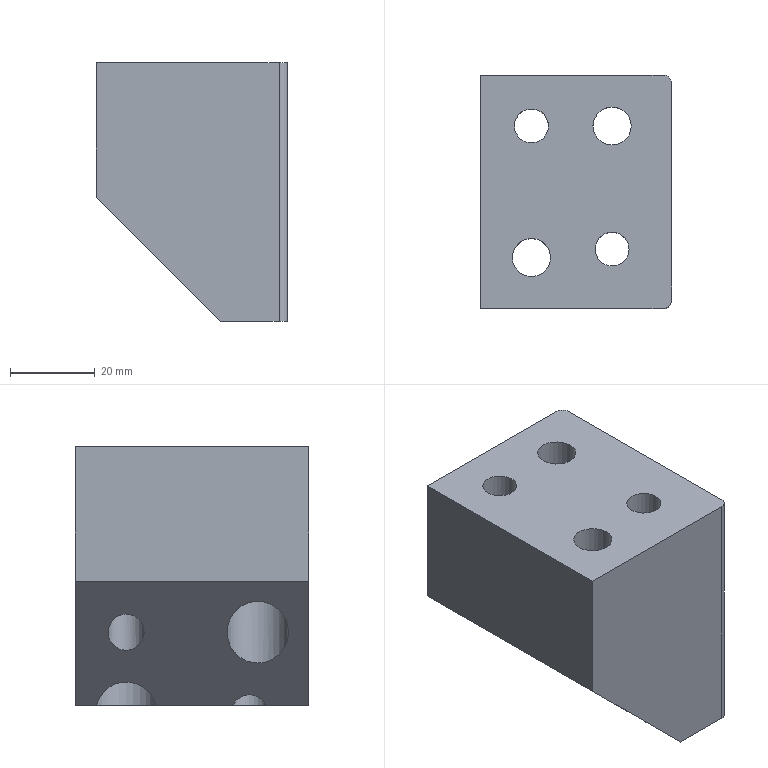Part | NX | features solid 2 | 1 solid | 21 faces | box 45 x 55 x 61 mm | volume 109585 mm3 | plane 11 | cylinder 10 | commonest cylinder face diameters 4 x2 8.001 x2 8.5 x2 9 x2 14.5 x2
STEP:
#1=CARTESIAN_POINT('',(620.135,-72.389,-6.));
#2=VERTEX_POINT('',#1);
#3=CARTESIAN_POINT('',(620.135,-80.141,-6.));
#4=VERTEX_POINT('',#3);
#5=CARTESIAN_POINT('',(621.878,-76.265,-6.));
#6=DIRECTION('',(0.,0.,1.));
#7=DIRECTION('',(1.,0.,0.));
#8=AXIS2_PLACEMENT_3D('',#5,#6,#7);
#9=CIRCLE('',#8,4.25);
#10=EDGE_CURVE('',#2,#4,#9,.F.);
#11=ORIENTED_EDGE('',*,*,#10,.F.);
#12=CARTESIAN_POINT('',(620.135,-54.303,-6.));
#13=VERTEX_POINT('',#12);
#14=CARTESIAN_POINT('',(620.135,88.864,-6.));
#15=DIRECTION('',(0.,1.,0.));
#16=VECTOR('',#15,1000.);
#17=LINE('',#14,#16);
#18=EDGE_CURVE('',#2,#13,#17,.T.);
#19=ORIENTED_EDGE('',*,*,#18,.T.);
#20=CARTESIAN_POINT('',(620.135,-40.228,-6.));
#21=VERTEX_POINT('',#20);
#22=CARTESIAN_POINT('',(621.878,-47.265,-6.));
#23=DIRECTION('',(0.,0.,-1.));
#24=DIRECTION('',(1.,0.,0.));
#25=AXIS2_PLACEMENT_3D('',#22,#23,#24);
#26=CIRCLE('',#25,7.25);
#27=EDGE_CURVE('',#13,#21,#26,.F.);
#28=ORIENTED_EDGE('',*,*,#27,.T.);
#29=CARTESIAN_POINT('',(620.135,-35.265,-6.));
#30=VERTEX_POINT('',#29);
#31=CARTESIAN_POINT('',(620.135,88.864,-6.));
#32=DIRECTION('',(0.,1.,0.));
#33=VECTOR('',#32,1000.);
#34=LINE('',#31,#33);
#35=EDGE_CURVE('',#21,#30,#34,.T.);
#36=ORIENTED_EDGE('',*,*,#35,.T.);
#37=CARTESIAN_POINT('',(633.878,-35.265,-6.));
#38=VERTEX_POINT('',#37);
#39=CARTESIAN_POINT('',(735.,-35.265,-6.));
#40=DIRECTION('',(-1.,0.,0.));
#41=VECTOR('',#40,1000.);
#42=LINE('',#39,#41);
#43=EDGE_CURVE('',#30,#38,#42,.F.);
#44=ORIENTED_EDGE('',*,*,#43,.T.);
#45=CARTESIAN_POINT('',(635.878,-37.265,-6.));
#46=VERTEX_POINT('',#45);
#47=CARTESIAN_POINT('',(633.878,-37.265,-6.));
#48=DIRECTION('',(0.,0.,1.));
#49=DIRECTION('',(1.,0.,0.));
#50=AXIS2_PLACEMENT_3D('',#47,#48,#49);
#51=CIRCLE('',#50,2.);
#52=EDGE_CURVE('',#46,#38,#51,.T.);
#53=ORIENTED_EDGE('',*,*,#52,.F.);
#54=CARTESIAN_POINT('',(635.878,-88.265,-6.));
#55=VERTEX_POINT('',#54);
#56=CARTESIAN_POINT('',(635.878,-52.29,-6.));
#57=DIRECTION('',(0.,1.,0.));
#58=VECTOR('',#57,1000.);
#59=LINE('',#56,#58);
#60=EDGE_CURVE('',#46,#55,#59,.F.);
#61=ORIENTED_EDGE('',*,*,#60,.T.);
#62=CARTESIAN_POINT('',(633.878,-90.265,-6.));
#63=VERTEX_POINT('',#62);
#64=CARTESIAN_POINT('',(633.878,-88.265,-6.));
#65=DIRECTION('',(0.,0.,1.));
#66=DIRECTION('',(1.,0.,0.));
#67=AXIS2_PLACEMENT_3D('',#64,#65,#66);
#68=CIRCLE('',#67,2.);
#69=EDGE_CURVE('',#55,#63,#68,.F.);
#70=ORIENTED_EDGE('',*,*,#69,.T.);
#71=CARTESIAN_POINT('',(620.135,-90.265,-6.));
#72=VERTEX_POINT('',#71);
#73=CARTESIAN_POINT('',(735.,-90.265,-6.));
#74=DIRECTION('',(1.,0.,0.));
#75=VECTOR('',#74,1000.);
#76=LINE('',#73,#75);
#77=EDGE_CURVE('',#63,#72,#76,.F.);
#78=ORIENTED_EDGE('',*,*,#77,.T.);
#79=CARTESIAN_POINT('',(620.135,88.864,-6.));
#80=DIRECTION('',(0.,1.,0.));
#81=VECTOR('',#80,1000.);
#82=LINE('',#79,#81);
#83=EDGE_CURVE('',#72,#4,#82,.T.);
#84=ORIENTED_EDGE('',*,*,#83,.T.);
#85=EDGE_LOOP('',(#11,#19,#28,#36,#44,#53,#61,#70,#78,#84));
#86=FACE_BOUND('',#85,.T.);
#87=CARTESIAN_POINT('',(735.,88.864,-6.));
#88=DIRECTION('',(0.,0.,1.));
#89=DIRECTION('',(-0.9997,0.02352,0.));
#90=AXIS2_PLACEMENT_3D('',#87,#88,#89);
#91=PLANE('',#90);
#92=ADVANCED_FACE('',(#86),#91,.F.);
#93=CARTESIAN_POINT('',(590.878,-90.265,23.257));
#94=VERTEX_POINT('',#93);
#95=CARTESIAN_POINT('',(590.878,-90.265,55.));
#96=VERTEX_POINT('',#95);
#97=CARTESIAN_POINT('',(590.878,-90.265,-5.));
#98=DIRECTION('',(0.,0.,1.));
#99=VECTOR('',#98,1000.);
#100=LINE('',#97,#99);
#101=EDGE_CURVE('',#94,#96,#100,.T.);
#102=ORIENTED_EDGE('',*,*,#101,.T.);
#103=CARTESIAN_POINT('',(590.878,-35.265,55.));
#104=VERTEX_POINT('',#103);
#105=CARTESIAN_POINT('',(590.878,-52.29,55.));
#106=DIRECTION('',(0.,1.,0.));
#107=VECTOR('',#106,1000.);
#108=LINE('',#105,#107);
#109=EDGE_CURVE('',#96,#104,#108,.T.);
#110=ORIENTED_EDGE('',*,*,#109,.T.);
#111=CARTESIAN_POINT('',(590.878,-35.265,23.257));
#112=VERTEX_POINT('',#111);
#113=CARTESIAN_POINT('',(590.878,-35.265,-5.));
#114=DIRECTION('',(0.,0.,1.));
#115=VECTOR('',#114,1000.);
#116=LINE('',#113,#115);
#117=EDGE_CURVE('',#112,#104,#116,.T.);
#118=ORIENTED_EDGE('',*,*,#117,.F.);
#119=CARTESIAN_POINT('',(590.878,-52.29,23.257));
#120=DIRECTION('',(0.,-1.,0.));
#121=VECTOR('',#120,1000.);
#122=LINE('',#119,#121);
#123=EDGE_CURVE('',#94,#112,#122,.F.);
#124=ORIENTED_EDGE('',*,*,#123,.F.);
#125=EDGE_LOOP('',(#102,#110,#118,#124));
#126=FACE_BOUND('',#125,.T.);
#127=CARTESIAN_POINT('',(590.878,-52.29,-5.));
#128=DIRECTION('',(-1.,0.,0.));
#129=DIRECTION('',(0.,0.,1.));
#130=AXIS2_PLACEMENT_3D('',#127,#128,#129);
#131=PLANE('',#130);
#132=ADVANCED_FACE('',(#126),#131,.T.);
#133=CARTESIAN_POINT('',(635.878,-37.265,55.));
#134=VERTEX_POINT('',#133);
#135=CARTESIAN_POINT('',(635.878,-37.265,-5.));
#136=DIRECTION('',(0.,0.,1.));
#137=VECTOR('',#136,1000.);
#138=LINE('',#135,#137);
#139=EDGE_CURVE('',#134,#46,#138,.F.);
#140=ORIENTED_EDGE('',*,*,#139,.F.);
#141=CARTESIAN_POINT('',(635.878,-88.265,55.));
#142=VERTEX_POINT('',#141);
#143=CARTESIAN_POINT('',(635.878,-52.29,55.));
#144=DIRECTION('',(0.,-1.,0.));
#145=VECTOR('',#144,1000.);
#146=LINE('',#143,#145);
#147=EDGE_CURVE('',#134,#142,#146,.T.);
#148=ORIENTED_EDGE('',*,*,#147,.T.);
#149=CARTESIAN_POINT('',(635.878,-88.265,-5.));
#150=DIRECTION('',(0.,0.,-1.));
#151=VECTOR('',#150,1000.);
#152=LINE('',#149,#151);
#153=EDGE_CURVE('',#142,#55,#152,.T.);
#154=ORIENTED_EDGE('',*,*,#153,.T.);
#155=ORIENTED_EDGE('',*,*,#60,.F.);
#156=EDGE_LOOP('',(#140,#148,#154,#155));
#157=FACE_BOUND('',#156,.T.);
#158=CARTESIAN_POINT('',(635.878,-52.29,-5.));
#159=DIRECTION('',(1.,0.,0.));
#160=DIRECTION('',(0.,0.,-1.));
#161=AXIS2_PLACEMENT_3D('',#158,#159,#160);
#162=PLANE('',#161);
#163=ADVANCED_FACE('',(#157),#162,.T.);
#164=ORIENTED_EDGE('',*,*,#117,.T.);
#165=CARTESIAN_POINT('',(633.878,-35.265,55.));
#166=VERTEX_POINT('',#165);
#167=CARTESIAN_POINT('',(630.878,-35.265,55.));
#168=DIRECTION('',(1.,0.,0.));
#169=VECTOR('',#168,1000.);
#170=LINE('',#167,#169);
#171=EDGE_CURVE('',#104,#166,#170,.T.);
#172=ORIENTED_EDGE('',*,*,#171,.T.);
#173=CARTESIAN_POINT('',(633.878,-35.265,-5.));
#174=DIRECTION('',(0.,0.,1.));
#175=VECTOR('',#174,1000.);
#176=LINE('',#173,#175);
#177=EDGE_CURVE('',#38,#166,#176,.T.);
#178=ORIENTED_EDGE('',*,*,#177,.F.);
#179=ORIENTED_EDGE('',*,*,#43,.F.);
#180=CARTESIAN_POINT('',(613.756,-35.265,0.3787));
#181=DIRECTION('',(-0.7071,0.,0.7071));
#182=VECTOR('',#181,1000.);
#183=LINE('',#180,#182);
#184=EDGE_CURVE('',#112,#30,#183,.F.);
#185=ORIENTED_EDGE('',*,*,#184,.F.);
#186=EDGE_LOOP('',(#164,#172,#178,#179,#185));
#187=FACE_BOUND('',#186,.T.);
#188=CARTESIAN_POINT('',(630.878,-35.265,-5.));
#189=DIRECTION('',(0.,1.,0.));
#190=DIRECTION('',(0.,0.,1.));
#191=AXIS2_PLACEMENT_3D('',#188,#189,#190);
#192=PLANE('',#191);
#193=ADVANCED_FACE('',(#187),#192,.T.);
#194=ORIENTED_EDGE('',*,*,#177,.T.);
#195=CARTESIAN_POINT('',(633.878,-37.265,55.));
#196=DIRECTION('',(0.,0.,1.));
#197=DIRECTION('',(1.,0.,0.));
#198=AXIS2_PLACEMENT_3D('',#195,#196,#197);
#199=CIRCLE('',#198,2.);
#200=EDGE_CURVE('',#166,#134,#199,.F.);
#201=ORIENTED_EDGE('',*,*,#200,.T.);
#202=ORIENTED_EDGE('',*,*,#139,.T.);
#203=ORIENTED_EDGE('',*,*,#52,.T.);
#204=EDGE_LOOP('',(#194,#201,#202,#203));
#205=FACE_BOUND('',#204,.T.);
#206=CARTESIAN_POINT('',(633.878,-37.265,-5.));
#207=DIRECTION('',(0.,0.,-1.));
#208=DIRECTION('',(-1.,0.,0.));
#209=AXIS2_PLACEMENT_3D('',#206,#207,#208);
#210=CYLINDRICAL_SURFACE('',#209,2.);
#211=ADVANCED_FACE('',(#205),#210,.T.);
#212=CARTESIAN_POINT('',(633.878,-90.265,55.));
#213=VERTEX_POINT('',#212);
#214=CARTESIAN_POINT('',(633.878,-90.265,22.));
#215=DIRECTION('',(0.,0.,-1.));
#216=VECTOR('',#215,1000.);
#217=LINE('',#214,#216);
#218=EDGE_CURVE('',#63,#213,#217,.F.);
#219=ORIENTED_EDGE('',*,*,#218,.T.);
#220=CARTESIAN_POINT('',(619.878,-90.265,55.));
#221=DIRECTION('',(-1.,0.,0.));
#222=VECTOR('',#221,1000.);
#223=LINE('',#220,#222);
#224=EDGE_CURVE('',#213,#96,#223,.T.);
#225=ORIENTED_EDGE('',*,*,#224,.T.);
#226=ORIENTED_EDGE('',*,*,#101,.F.);
#227=CARTESIAN_POINT('',(613.756,-90.265,0.3787));
#228=DIRECTION('',(0.7071,0.,-0.7071));
#229=VECTOR('',#228,1000.);
#230=LINE('',#227,#229);
#231=EDGE_CURVE('',#72,#94,#230,.F.);
#232=ORIENTED_EDGE('',*,*,#231,.F.);
#233=ORIENTED_EDGE('',*,*,#77,.F.);
#234=EDGE_LOOP('',(#219,#225,#226,#232,#233));
#235=FACE_BOUND('',#234,.T.);
#236=CARTESIAN_POINT('',(619.878,-90.265,22.));
#237=DIRECTION('',(0.,-1.,0.));
#238=DIRECTION('',(0.,0.,-1.));
#239=AXIS2_PLACEMENT_3D('',#236,#237,#238);
#240=PLANE('',#239);
#241=ADVANCED_FACE('',(#235),#240,.T.);
#242=ORIENTED_EDGE('',*,*,#153,.F.);
#243=CARTESIAN_POINT('',(633.878,-88.265,55.));
#244=DIRECTION('',(0.,0.,1.));
#245=DIRECTION('',(1.,0.,0.));
#246=AXIS2_PLACEMENT_3D('',#243,#244,#245);
#247=CIRCLE('',#246,2.);
#248=EDGE_CURVE('',#142,#213,#247,.F.);
#249=ORIENTED_EDGE('',*,*,#248,.T.);
#250=ORIENTED_EDGE('',*,*,#218,.F.);
#251=ORIENTED_EDGE('',*,*,#69,.F.);
#252=EDGE_LOOP('',(#242,#249,#250,#251));
#253=FACE_BOUND('',#252,.T.);
#254=CARTESIAN_POINT('',(633.878,-88.265,-5.));
#255=DIRECTION('',(0.,0.,-1.));
#256=DIRECTION('',(-1.,0.,0.));
#257=AXIS2_PLACEMENT_3D('',#254,#255,#256);
#258=CYLINDRICAL_SURFACE('',#257,2.);
#259=ADVANCED_FACE('',(#253),#258,.T.);
#260=CARTESIAN_POINT('',(598.628,-47.265,15.507));
#261=VERTEX_POINT('',#260);
#262=CARTESIAN_POINT('',(602.878,-47.265,11.257));
#263=DIRECTION('',(0.7071,0.,0.7071));
#264=DIRECTION('',(-0.7071,0.,0.7071));
#265=AXIS2_PLACEMENT_3D('',#262,#263,#264);
#266=ELLIPSE('',#265,6.01,4.25);
#267=EDGE_CURVE('',#261,#261,#266,.F.);
#268=ORIENTED_EDGE('',*,*,#267,.F.);
#269=EDGE_LOOP('',(#268));
#270=FACE_BOUND('',#269,.T.);
#271=CARTESIAN_POINT('',(621.878,-76.265,-7.743));
#272=DIRECTION('',(0.7071,0.,0.7071));
#273=DIRECTION('',(-0.7071,0.,0.7071));
#274=AXIS2_PLACEMENT_3D('',#271,#272,#273);
#275=ELLIPSE('',#274,6.01,4.25);
#276=EDGE_CURVE('',#4,#2,#275,.F.);
#277=ORIENTED_EDGE('',*,*,#276,.F.);
#278=ORIENTED_EDGE('',*,*,#83,.F.);
#279=ORIENTED_EDGE('',*,*,#231,.T.);
#280=ORIENTED_EDGE('',*,*,#123,.T.);
#281=ORIENTED_EDGE('',*,*,#184,.T.);
#282=ORIENTED_EDGE('',*,*,#35,.F.);
#283=CARTESIAN_POINT('',(621.878,-47.265,-7.743));
#284=DIRECTION('',(0.7071,0.,0.7071));
#285=DIRECTION('',(-0.7071,0.,0.7071));
#286=AXIS2_PLACEMENT_3D('',#283,#284,#285);
#287=ELLIPSE('',#286,10.253,7.25);
#288=EDGE_CURVE('',#13,#21,#287,.F.);
#289=ORIENTED_EDGE('',*,*,#288,.F.);
#290=ORIENTED_EDGE('',*,*,#18,.F.);
#291=EDGE_LOOP('',(#277,#278,#279,#280,#281,#282,#289,#290));
#292=FACE_BOUND('',#291,.T.);
#293=CARTESIAN_POINT('',(595.628,-78.265,18.507));
#294=VERTEX_POINT('',#293);
#295=CARTESIAN_POINT('',(602.878,-78.265,11.257));
#296=DIRECTION('',(0.7071,0.,0.7071));
#297=DIRECTION('',(-0.7071,0.,0.7071));
#298=AXIS2_PLACEMENT_3D('',#295,#296,#297);
#299=ELLIPSE('',#298,10.253,7.25);
#300=EDGE_CURVE('',#294,#294,#299,.F.);
#301=ORIENTED_EDGE('',*,*,#300,.F.);
#302=EDGE_LOOP('',(#301));
#303=FACE_BOUND('',#302,.T.);
#304=CARTESIAN_POINT('',(613.756,-52.29,0.3787));
#305=DIRECTION('',(0.7071,0.,0.7071));
#306=DIRECTION('',(0.,1.,0.));
#307=AXIS2_PLACEMENT_3D('',#304,#305,#306);
#308=PLANE('',#307);
#309=ADVANCED_FACE('',(#270,#292,#303),#308,.F.);
#310=CARTESIAN_POINT('',(606.878,-47.265,55.));
#311=VERTEX_POINT('',#310);
#312=CARTESIAN_POINT('',(602.878,-47.265,55.));
#313=DIRECTION('',(0.,0.,1.));
#314=DIRECTION('',(1.,0.,0.));
#315=AXIS2_PLACEMENT_3D('',#312,#313,#314);
#316=CIRCLE('',#315,4.);
#317=EDGE_CURVE('',#311,#311,#316,.T.);
#318=ORIENTED_EDGE('',*,*,#317,.F.);
#319=EDGE_LOOP('',(#318));
#320=FACE_BOUND('',#319,.T.);
#321=CARTESIAN_POINT('',(625.878,-76.265,55.));
#322=VERTEX_POINT('',#321);
#323=CARTESIAN_POINT('',(621.878,-76.265,55.));
#324=DIRECTION('',(0.,0.,1.));
#325=DIRECTION('',(1.,0.,0.));
#326=AXIS2_PLACEMENT_3D('',#323,#324,#325);
#327=CIRCLE('',#326,4.);
#328=EDGE_CURVE('',#322,#322,#327,.T.);
#329=ORIENTED_EDGE('',*,*,#328,.F.);
#330=EDGE_LOOP('',(#329));
#331=FACE_BOUND('',#330,.T.);
#332=CARTESIAN_POINT('',(626.378,-47.265,55.));
#333=VERTEX_POINT('',#332);
#334=CARTESIAN_POINT('',(621.878,-47.265,55.));
#335=DIRECTION('',(0.,0.,1.));
#336=DIRECTION('',(1.,0.,0.));
#337=AXIS2_PLACEMENT_3D('',#334,#335,#336);
#338=CIRCLE('',#337,4.5);
#339=EDGE_CURVE('',#333,#333,#338,.T.);
#340=ORIENTED_EDGE('',*,*,#339,.F.);
#341=EDGE_LOOP('',(#340));
#342=FACE_BOUND('',#341,.T.);
#343=CARTESIAN_POINT('',(607.378,-78.265,55.));
#344=VERTEX_POINT('',#343);
#345=CARTESIAN_POINT('',(602.878,-78.265,55.));
#346=DIRECTION('',(0.,0.,1.));
#347=DIRECTION('',(1.,0.,0.));
#348=AXIS2_PLACEMENT_3D('',#345,#346,#347);
#349=CIRCLE('',#348,4.5);
#350=EDGE_CURVE('',#344,#344,#349,.T.);
#351=ORIENTED_EDGE('',*,*,#350,.F.);
#352=EDGE_LOOP('',(#351));
#353=FACE_BOUND('',#352,.T.);
#354=ORIENTED_EDGE('',*,*,#171,.F.);
#355=ORIENTED_EDGE('',*,*,#109,.F.);
#356=ORIENTED_EDGE('',*,*,#224,.F.);
#357=ORIENTED_EDGE('',*,*,#248,.F.);
#358=ORIENTED_EDGE('',*,*,#147,.F.);
#359=ORIENTED_EDGE('',*,*,#200,.F.);
#360=EDGE_LOOP('',(#354,#355,#356,#357,#358,#359));
#361=FACE_BOUND('',#360,.T.);
#362=CARTESIAN_POINT('',(612.,0.,55.));
#363=DIRECTION('',(0.,0.,1.));
#364=DIRECTION('',(1.,0.,0.));
#365=AXIS2_PLACEMENT_3D('',#362,#363,#364);
#366=PLANE('',#365);
#367=ADVANCED_FACE('',(#320,#331,#342,#353,#361),#366,.T.);
#368=ORIENTED_EDGE('',*,*,#350,.T.);
#369=EDGE_LOOP('',(#368));
#370=FACE_BOUND('',#369,.T.);
#371=CARTESIAN_POINT('',(598.378,-78.265,30.));
#372=VERTEX_POINT('',#371);
#373=CARTESIAN_POINT('',(602.878,-78.265,30.));
#374=DIRECTION('',(0.,0.,-1.));
#375=DIRECTION('',(-1.,0.,0.));
#376=AXIS2_PLACEMENT_3D('',#373,#374,#375);
#377=CIRCLE('',#376,4.5);
#378=EDGE_CURVE('',#372,#372,#377,.F.);
#379=ORIENTED_EDGE('',*,*,#378,.F.);
#380=EDGE_LOOP('',(#379));
#381=FACE_BOUND('',#380,.T.);
#382=CARTESIAN_POINT('',(602.878,-78.265,-8.));
#383=DIRECTION('',(0.,0.,1.));
#384=DIRECTION('',(1.,0.,0.));
#385=AXIS2_PLACEMENT_3D('',#382,#383,#384);
#386=CYLINDRICAL_SURFACE('',#385,4.5);
#387=ADVANCED_FACE('',(#370,#381),#386,.F.);
#388=ORIENTED_EDGE('',*,*,#378,.T.);
#389=EDGE_LOOP('',(#388));
#390=FACE_BOUND('',#389,.T.);
#391=CARTESIAN_POINT('',(610.128,-78.265,30.));
#392=VERTEX_POINT('',#391);
#393=CARTESIAN_POINT('',(602.878,-78.265,30.));
#394=DIRECTION('',(0.,0.,1.));
#395=DIRECTION('',(1.,0.,0.));
#396=AXIS2_PLACEMENT_3D('',#393,#394,#395);
#397=CIRCLE('',#396,7.25);
#398=EDGE_CURVE('',#392,#392,#397,.T.);
#399=ORIENTED_EDGE('',*,*,#398,.F.);
#400=EDGE_LOOP('',(#399));
#401=FACE_BOUND('',#400,.T.);
#402=CARTESIAN_POINT('',(602.878,-78.265,30.));
#403=DIRECTION('',(0.,0.,1.));
#404=DIRECTION('',(-1.,0.,0.));
#405=AXIS2_PLACEMENT_3D('',#402,#403,#404);
#406=PLANE('',#405);
#407=ADVANCED_FACE('',(#390,#401),#406,.F.);
#408=ORIENTED_EDGE('',*,*,#300,.T.);
#409=EDGE_LOOP('',(#408));
#410=FACE_BOUND('',#409,.T.);
#411=ORIENTED_EDGE('',*,*,#398,.T.);
#412=EDGE_LOOP('',(#411));
#413=FACE_BOUND('',#412,.T.);
#414=CARTESIAN_POINT('',(602.878,-78.265,-6.));
#415=DIRECTION('',(0.,0.,1.));
#416=DIRECTION('',(1.,0.,0.));
#417=AXIS2_PLACEMENT_3D('',#414,#415,#416);
#418=CYLINDRICAL_SURFACE('',#417,7.25);
#419=ADVANCED_FACE('',(#410,#413),#418,.F.);
#420=ORIENTED_EDGE('',*,*,#339,.T.);
#421=EDGE_LOOP('',(#420));
#422=FACE_BOUND('',#421,.T.);
#423=CARTESIAN_POINT('',(617.378,-47.265,30.));
#424=VERTEX_POINT('',#423);
#425=CARTESIAN_POINT('',(621.878,-47.265,30.));
#426=DIRECTION('',(0.,0.,-1.));
#427=DIRECTION('',(-1.,0.,0.));
#428=AXIS2_PLACEMENT_3D('',#425,#426,#427);
#429=CIRCLE('',#428,4.5);
#430=EDGE_CURVE('',#424,#424,#429,.F.);
#431=ORIENTED_EDGE('',*,*,#430,.F.);
#432=EDGE_LOOP('',(#431));
#433=FACE_BOUND('',#432,.T.);
#434=CARTESIAN_POINT('',(621.878,-47.265,-8.));
#435=DIRECTION('',(0.,0.,1.));
#436=DIRECTION('',(1.,0.,0.));
#437=AXIS2_PLACEMENT_3D('',#434,#435,#436);
#438=CYLINDRICAL_SURFACE('',#437,4.5);
#439=ADVANCED_FACE('',(#422,#433),#438,.F.);
#440=ORIENTED_EDGE('',*,*,#430,.T.);
#441=EDGE_LOOP('',(#440));
#442=FACE_BOUND('',#441,.T.);
#443=CARTESIAN_POINT('',(629.128,-47.265,30.));
#444=VERTEX_POINT('',#443);
#445=CARTESIAN_POINT('',(621.878,-47.265,30.));
#446=DIRECTION('',(0.,0.,1.));
#447=DIRECTION('',(1.,0.,0.));
#448=AXIS2_PLACEMENT_3D('',#445,#446,#447);
#449=CIRCLE('',#448,7.25);
#450=EDGE_CURVE('',#444,#444,#449,.T.);
#451=ORIENTED_EDGE('',*,*,#450,.F.);
#452=EDGE_LOOP('',(#451));
#453=FACE_BOUND('',#452,.T.);
#454=CARTESIAN_POINT('',(621.878,-47.265,30.));
#455=DIRECTION('',(0.,0.,1.));
#456=DIRECTION('',(-1.,0.,0.));
#457=AXIS2_PLACEMENT_3D('',#454,#455,#456);
#458=PLANE('',#457);
#459=ADVANCED_FACE('',(#442,#453),#458,.F.);
#460=ORIENTED_EDGE('',*,*,#288,.T.);
#461=ORIENTED_EDGE('',*,*,#27,.F.);
#462=EDGE_LOOP('',(#460,#461));
#463=FACE_BOUND('',#462,.T.);
#464=ORIENTED_EDGE('',*,*,#450,.T.);
#465=EDGE_LOOP('',(#464));
#466=FACE_BOUND('',#465,.T.);
#467=CARTESIAN_POINT('',(621.878,-47.265,-6.));
#468=DIRECTION('',(0.,0.,1.));
#469=DIRECTION('',(1.,0.,0.));
#470=AXIS2_PLACEMENT_3D('',#467,#468,#469);
#471=CYLINDRICAL_SURFACE('',#470,7.25);
#472=ADVANCED_FACE('',(#463,#466),#471,.F.);
#473=ORIENTED_EDGE('',*,*,#328,.T.);
#474=EDGE_LOOP('',(#473));
#475=FACE_BOUND('',#474,.T.);
#476=CARTESIAN_POINT('',(617.877,-76.265,34.));
#477=VERTEX_POINT('',#476);
#478=CARTESIAN_POINT('',(621.878,-76.265,34.));
#479=DIRECTION('',(0.,0.,-1.));
#480=DIRECTION('',(-1.,0.,0.));
#481=AXIS2_PLACEMENT_3D('',#478,#479,#480);
#482=CIRCLE('',#481,4.);
#483=EDGE_CURVE('',#477,#477,#482,.F.);
#484=ORIENTED_EDGE('',*,*,#483,.F.);
#485=EDGE_LOOP('',(#484));
#486=FACE_BOUND('',#485,.T.);
#487=CARTESIAN_POINT('',(621.878,-76.265,-8.));
#488=DIRECTION('',(0.,0.,1.));
#489=DIRECTION('',(1.,0.,0.));
#490=AXIS2_PLACEMENT_3D('',#487,#488,#489);
#491=CYLINDRICAL_SURFACE('',#490,4.);
#492=ADVANCED_FACE('',(#475,#486),#491,.F.);
#493=ORIENTED_EDGE('',*,*,#483,.T.);
#494=EDGE_LOOP('',(#493));
#495=FACE_BOUND('',#494,.T.);
#496=CARTESIAN_POINT('',(626.128,-76.265,34.));
#497=VERTEX_POINT('',#496);
#498=CARTESIAN_POINT('',(621.878,-76.265,34.));
#499=DIRECTION('',(0.,0.,1.));
#500=DIRECTION('',(1.,0.,0.));
#501=AXIS2_PLACEMENT_3D('',#498,#499,#500);
#502=CIRCLE('',#501,4.25);
#503=EDGE_CURVE('',#497,#497,#502,.T.);
#504=ORIENTED_EDGE('',*,*,#503,.F.);
#505=EDGE_LOOP('',(#504));
#506=FACE_BOUND('',#505,.T.);
#507=CARTESIAN_POINT('',(621.878,-76.265,34.));
#508=DIRECTION('',(0.,0.,1.));
#509=DIRECTION('',(-1.,0.,0.));
#510=AXIS2_PLACEMENT_3D('',#507,#508,#509);
#511=PLANE('',#510);
#512=ADVANCED_FACE('',(#495,#506),#511,.F.);
#513=ORIENTED_EDGE('',*,*,#10,.T.);
#514=ORIENTED_EDGE('',*,*,#276,.T.);
#515=EDGE_LOOP('',(#513,#514));
#516=FACE_BOUND('',#515,.T.);
#517=ORIENTED_EDGE('',*,*,#503,.T.);
#518=EDGE_LOOP('',(#517));
#519=FACE_BOUND('',#518,.T.);
#520=CARTESIAN_POINT('',(621.878,-76.265,-8.));
#521=DIRECTION('',(0.,0.,1.));
#522=DIRECTION('',(1.,0.,0.));
#523=AXIS2_PLACEMENT_3D('',#520,#521,#522);
#524=CYLINDRICAL_SURFACE('',#523,4.25);
#525=ADVANCED_FACE('',(#516,#519),#524,.F.);
#526=ORIENTED_EDGE('',*,*,#317,.T.);
#527=EDGE_LOOP('',(#526));
#528=FACE_BOUND('',#527,.T.);
#529=CARTESIAN_POINT('',(598.877,-47.265,34.));
#530=VERTEX_POINT('',#529);
#531=CARTESIAN_POINT('',(602.878,-47.265,34.));
#532=DIRECTION('',(0.,0.,-1.));
#533=DIRECTION('',(-1.,0.,0.));
#534=AXIS2_PLACEMENT_3D('',#531,#532,#533);
#535=CIRCLE('',#534,4.);
#536=EDGE_CURVE('',#530,#530,#535,.F.);
#537=ORIENTED_EDGE('',*,*,#536,.F.);
#538=EDGE_LOOP('',(#537));
#539=FACE_BOUND('',#538,.T.);
#540=CARTESIAN_POINT('',(602.878,-47.265,-8.));
#541=DIRECTION('',(0.,0.,1.));
#542=DIRECTION('',(1.,0.,0.));
#543=AXIS2_PLACEMENT_3D('',#540,#541,#542);
#544=CYLINDRICAL_SURFACE('',#543,4.);
#545=ADVANCED_FACE('',(#528,#539),#544,.F.);
#546=ORIENTED_EDGE('',*,*,#536,.T.);
#547=EDGE_LOOP('',(#546));
#548=FACE_BOUND('',#547,.T.);
#549=CARTESIAN_POINT('',(607.128,-47.265,34.));
#550=VERTEX_POINT('',#549);
#551=CARTESIAN_POINT('',(602.878,-47.265,34.));
#552=DIRECTION('',(0.,0.,1.));
#553=DIRECTION('',(1.,0.,0.));
#554=AXIS2_PLACEMENT_3D('',#551,#552,#553);
#555=CIRCLE('',#554,4.25);
#556=EDGE_CURVE('',#550,#550,#555,.T.);
#557=ORIENTED_EDGE('',*,*,#556,.F.);
#558=EDGE_LOOP('',(#557));
#559=FACE_BOUND('',#558,.T.);
#560=CARTESIAN_POINT('',(602.878,-47.265,34.));
#561=DIRECTION('',(0.,0.,1.));
#562=DIRECTION('',(-1.,0.,0.));
#563=AXIS2_PLACEMENT_3D('',#560,#561,#562);
#564=PLANE('',#563);
#565=ADVANCED_FACE('',(#548,#559),#564,.F.);
#566=ORIENTED_EDGE('',*,*,#267,.T.);
#567=EDGE_LOOP('',(#566));
#568=FACE_BOUND('',#567,.T.);
#569=ORIENTED_EDGE('',*,*,#556,.T.);
#570=EDGE_LOOP('',(#569));
#571=FACE_BOUND('',#570,.T.);
#572=CARTESIAN_POINT('',(602.878,-47.265,-8.));
#573=DIRECTION('',(0.,0.,1.));
#574=DIRECTION('',(1.,0.,0.));
#575=AXIS2_PLACEMENT_3D('',#572,#573,#574);
#576=CYLINDRICAL_SURFACE('',#575,4.25);
#577=ADVANCED_FACE('',(#568,#571),#576,.F.);
#578=CLOSED_SHELL('',(#92,#132,#163,#193,#211,#241,#259,#309,#367,#387,#407,#419,#439,#459,#472,#492,#512,#525,#545,#565,#577));
#579=MANIFOLD_SOLID_BREP('',#578);
#580=(LENGTH_UNIT()NAMED_UNIT(*)SI_UNIT(.MILLI.,.METRE.));
#581=UNCERTAINTY_MEASURE_WITH_UNIT(LENGTH_MEASURE(0.00001),#580,'','');
#582=(NAMED_UNIT(*)PLANE_ANGLE_UNIT()SI_UNIT($,.RADIAN.));
#583=(NAMED_UNIT(*)SI_UNIT($,.STERADIAN.)SOLID_ANGLE_UNIT());
#584=(GEOMETRIC_REPRESENTATION_CONTEXT(3)GLOBAL_UNCERTAINTY_ASSIGNED_CONTEXT((#581))GLOBAL_UNIT_ASSIGNED_CONTEXT((#580,#582,#583))REPRESENTATION_CONTEXT('',''));
#585=ADVANCED_BREP_SHAPE_REPRESENTATION('',(#579),#584);